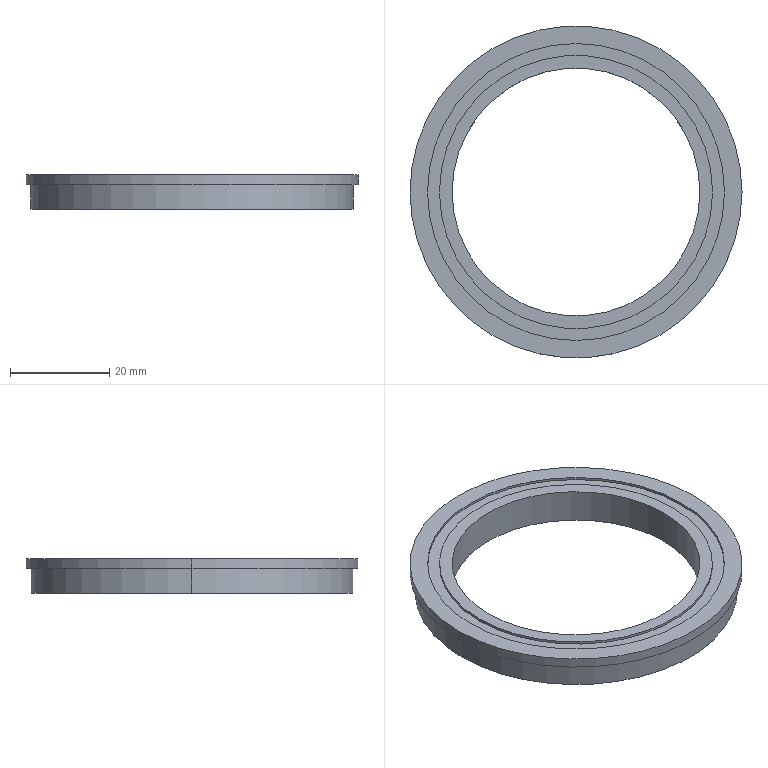Part | SolidWorks | features ICE 1, Revolution 1 | 1 solid | 21 faces | box 67 x 67 x 7 mm | volume 9465 mm3 | cylinder 14 | plane 7 | commonest cylinder face diameters 55.1 x4 59.9 x4 50 x2 65 x2 67 x2
STEP:
#1=CARTESIAN_POINT('',(33.5,0.,1.5));
#2=VERTEX_POINT('',#1);
#3=CARTESIAN_POINT('',(-33.5,0.,1.5));
#4=VERTEX_POINT('',#3);
#5=CARTESIAN_POINT('',(0.,0.,1.5));
#6=DIRECTION('',(0.,0.,1.));
#7=DIRECTION('',(1.,0.,0.));
#8=AXIS2_PLACEMENT_3D('',#5,#6,#7);
#9=CIRCLE('',#8,33.5);
#10=EDGE_CURVE('',#2,#4,#9,.T.);
#11=ORIENTED_EDGE('',*,*,#10,.T.);
#12=CARTESIAN_POINT('',(-33.5,0.,3.5));
#13=VERTEX_POINT('',#12);
#14=CARTESIAN_POINT('',(-33.5,0.,1.5));
#15=DIRECTION('',(0.,0.,1.));
#16=VECTOR('',#15,1000.);
#17=LINE('',#14,#16);
#18=EDGE_CURVE('',#4,#13,#17,.T.);
#19=ORIENTED_EDGE('',*,*,#18,.T.);
#20=CARTESIAN_POINT('',(33.5,0.,3.5));
#21=VERTEX_POINT('',#20);
#22=CARTESIAN_POINT('',(0.,0.,3.5));
#23=DIRECTION('',(0.,0.,1.));
#24=DIRECTION('',(1.,0.,0.));
#25=AXIS2_PLACEMENT_3D('',#22,#23,#24);
#26=CIRCLE('',#25,33.5);
#27=EDGE_CURVE('',#21,#13,#26,.T.);
#28=ORIENTED_EDGE('',*,*,#27,.F.);
#29=CARTESIAN_POINT('',(33.5,0.,1.5));
#30=DIRECTION('',(0.,0.,1.));
#31=VECTOR('',#30,1000.);
#32=LINE('',#29,#31);
#33=EDGE_CURVE('',#2,#21,#32,.T.);
#34=ORIENTED_EDGE('',*,*,#33,.F.);
#35=EDGE_LOOP('',(#11,#19,#28,#34));
#36=FACE_OUTER_BOUND('',#35,.T.);
#37=CARTESIAN_POINT('',(0.,0.,1.5));
#38=DIRECTION('',(0.,0.,1.));
#39=DIRECTION('',(1.,0.,0.));
#40=AXIS2_PLACEMENT_3D('',#37,#38,#39);
#41=CYLINDRICAL_SURFACE('',#40,33.5);
#42=ADVANCED_FACE('',(#36),#41,.T.);
#43=CARTESIAN_POINT('',(27.55,0.,-3.5));
#44=VERTEX_POINT('',#43);
#45=CARTESIAN_POINT('',(-27.55,0.,-3.5));
#46=VERTEX_POINT('',#45);
#47=CARTESIAN_POINT('',(0.,0.,-3.5));
#48=DIRECTION('',(0.,0.,1.));
#49=DIRECTION('',(1.,0.,0.));
#50=AXIS2_PLACEMENT_3D('',#47,#48,#49);
#51=CIRCLE('',#50,27.55);
#52=EDGE_CURVE('',#44,#46,#51,.T.);
#53=ORIENTED_EDGE('',*,*,#52,.T.);
#54=CARTESIAN_POINT('',(-27.55,0.,-3.));
#55=VERTEX_POINT('',#54);
#56=CARTESIAN_POINT('',(-27.55,0.,0.));
#57=DIRECTION('',(0.,0.,1.));
#58=VECTOR('',#57,1000.);
#59=LINE('',#56,#58);
#60=EDGE_CURVE('',#46,#55,#59,.T.);
#61=ORIENTED_EDGE('',*,*,#60,.T.);
#62=CARTESIAN_POINT('',(27.55,0.,-3.));
#63=VERTEX_POINT('',#62);
#64=CARTESIAN_POINT('',(0.,0.,-3.));
#65=DIRECTION('',(0.,0.,1.));
#66=DIRECTION('',(1.,0.,0.));
#67=AXIS2_PLACEMENT_3D('',#64,#65,#66);
#68=CIRCLE('',#67,27.55);
#69=EDGE_CURVE('',#63,#55,#68,.T.);
#70=ORIENTED_EDGE('',*,*,#69,.F.);
#71=CARTESIAN_POINT('',(27.55,0.,0.));
#72=DIRECTION('',(0.,0.,1.));
#73=VECTOR('',#72,1000.);
#74=LINE('',#71,#73);
#75=EDGE_CURVE('',#44,#63,#74,.T.);
#76=ORIENTED_EDGE('',*,*,#75,.F.);
#77=EDGE_LOOP('',(#53,#61,#70,#76));
#78=FACE_OUTER_BOUND('',#77,.T.);
#79=CARTESIAN_POINT('',(0.,0.,0.));
#80=DIRECTION('',(0.,0.,1.));
#81=DIRECTION('',(1.,0.,0.));
#82=AXIS2_PLACEMENT_3D('',#79,#80,#81);
#83=CYLINDRICAL_SURFACE('',#82,27.55);
#84=ADVANCED_FACE('',(#78),#83,.T.);
#85=CARTESIAN_POINT('',(-29.95,0.,-3.5));
#86=VERTEX_POINT('',#85);
#87=CARTESIAN_POINT('',(29.95,0.,-3.5));
#88=VERTEX_POINT('',#87);
#89=CARTESIAN_POINT('',(0.,0.,-3.5));
#90=DIRECTION('',(0.,0.,1.));
#91=DIRECTION('',(1.,0.,0.));
#92=AXIS2_PLACEMENT_3D('',#89,#90,#91);
#93=CIRCLE('',#92,29.95);
#94=EDGE_CURVE('',#86,#88,#93,.T.);
#95=ORIENTED_EDGE('',*,*,#94,.F.);
#96=CARTESIAN_POINT('',(-29.95,0.,-3.));
#97=VERTEX_POINT('',#96);
#98=CARTESIAN_POINT('',(-29.95,0.,0.));
#99=DIRECTION('',(0.,0.,1.));
#100=VECTOR('',#99,1000.);
#101=LINE('',#98,#100);
#102=EDGE_CURVE('',#86,#97,#101,.T.);
#103=ORIENTED_EDGE('',*,*,#102,.T.);
#104=CARTESIAN_POINT('',(29.95,0.,-3.));
#105=VERTEX_POINT('',#104);
#106=CARTESIAN_POINT('',(0.,0.,-3.));
#107=DIRECTION('',(0.,0.,1.));
#108=DIRECTION('',(1.,0.,0.));
#109=AXIS2_PLACEMENT_3D('',#106,#107,#108);
#110=CIRCLE('',#109,29.95);
#111=EDGE_CURVE('',#97,#105,#110,.T.);
#112=ORIENTED_EDGE('',*,*,#111,.T.);
#113=CARTESIAN_POINT('',(29.95,0.,0.));
#114=DIRECTION('',(0.,0.,1.));
#115=VECTOR('',#114,1000.);
#116=LINE('',#113,#115);
#117=EDGE_CURVE('',#88,#105,#116,.T.);
#118=ORIENTED_EDGE('',*,*,#117,.F.);
#119=EDGE_LOOP('',(#95,#103,#112,#118));
#120=FACE_OUTER_BOUND('',#119,.T.);
#121=CARTESIAN_POINT('',(0.,0.,0.));
#122=DIRECTION('',(0.,0.,1.));
#123=DIRECTION('',(1.,0.,0.));
#124=AXIS2_PLACEMENT_3D('',#121,#122,#123);
#125=CYLINDRICAL_SURFACE('',#124,29.95);
#126=ADVANCED_FACE('',(#120),#125,.F.);
#127=CARTESIAN_POINT('',(-29.95,0.,3.));
#128=VERTEX_POINT('',#127);
#129=CARTESIAN_POINT('',(29.95,0.,3.));
#130=VERTEX_POINT('',#129);
#131=CARTESIAN_POINT('',(0.,0.,3.));
#132=DIRECTION('',(0.,0.,1.));
#133=DIRECTION('',(1.,0.,0.));
#134=AXIS2_PLACEMENT_3D('',#131,#132,#133);
#135=CIRCLE('',#134,29.95);
#136=EDGE_CURVE('',#128,#130,#135,.T.);
#137=ORIENTED_EDGE('',*,*,#136,.F.);
#138=CARTESIAN_POINT('',(-29.95,0.,3.5));
#139=VERTEX_POINT('',#138);
#140=CARTESIAN_POINT('',(-29.95,0.,0.));
#141=DIRECTION('',(0.,0.,1.));
#142=VECTOR('',#141,1000.);
#143=LINE('',#140,#142);
#144=EDGE_CURVE('',#128,#139,#143,.T.);
#145=ORIENTED_EDGE('',*,*,#144,.T.);
#146=CARTESIAN_POINT('',(29.95,0.,3.5));
#147=VERTEX_POINT('',#146);
#148=CARTESIAN_POINT('',(0.,0.,3.5));
#149=DIRECTION('',(0.,0.,1.));
#150=DIRECTION('',(1.,0.,0.));
#151=AXIS2_PLACEMENT_3D('',#148,#149,#150);
#152=CIRCLE('',#151,29.95);
#153=EDGE_CURVE('',#139,#147,#152,.T.);
#154=ORIENTED_EDGE('',*,*,#153,.T.);
#155=CARTESIAN_POINT('',(29.95,0.,0.));
#156=DIRECTION('',(0.,0.,1.));
#157=VECTOR('',#156,1000.);
#158=LINE('',#155,#157);
#159=EDGE_CURVE('',#130,#147,#158,.T.);
#160=ORIENTED_EDGE('',*,*,#159,.F.);
#161=EDGE_LOOP('',(#137,#145,#154,#160));
#162=FACE_OUTER_BOUND('',#161,.T.);
#163=CARTESIAN_POINT('',(0.,0.,0.));
#164=DIRECTION('',(0.,0.,1.));
#165=DIRECTION('',(1.,0.,0.));
#166=AXIS2_PLACEMENT_3D('',#163,#164,#165);
#167=CYLINDRICAL_SURFACE('',#166,29.95);
#168=ADVANCED_FACE('',(#162),#167,.F.);
#169=CARTESIAN_POINT('',(27.55,0.,3.));
#170=VERTEX_POINT('',#169);
#171=CARTESIAN_POINT('',(-27.55,0.,3.));
#172=VERTEX_POINT('',#171);
#173=CARTESIAN_POINT('',(0.,0.,3.));
#174=DIRECTION('',(0.,0.,1.));
#175=DIRECTION('',(1.,0.,0.));
#176=AXIS2_PLACEMENT_3D('',#173,#174,#175);
#177=CIRCLE('',#176,27.55);
#178=EDGE_CURVE('',#170,#172,#177,.T.);
#179=ORIENTED_EDGE('',*,*,#178,.T.);
#180=CARTESIAN_POINT('',(-27.55,0.,3.5));
#181=VERTEX_POINT('',#180);
#182=CARTESIAN_POINT('',(-27.55,0.,0.));
#183=DIRECTION('',(0.,0.,1.));
#184=VECTOR('',#183,1000.);
#185=LINE('',#182,#184);
#186=EDGE_CURVE('',#172,#181,#185,.T.);
#187=ORIENTED_EDGE('',*,*,#186,.T.);
#188=CARTESIAN_POINT('',(27.55,0.,3.5));
#189=VERTEX_POINT('',#188);
#190=CARTESIAN_POINT('',(0.,0.,3.5));
#191=DIRECTION('',(0.,0.,1.));
#192=DIRECTION('',(1.,0.,0.));
#193=AXIS2_PLACEMENT_3D('',#190,#191,#192);
#194=CIRCLE('',#193,27.55);
#195=EDGE_CURVE('',#189,#181,#194,.T.);
#196=ORIENTED_EDGE('',*,*,#195,.F.);
#197=CARTESIAN_POINT('',(27.55,0.,0.));
#198=DIRECTION('',(0.,0.,1.));
#199=VECTOR('',#198,1000.);
#200=LINE('',#197,#199);
#201=EDGE_CURVE('',#170,#189,#200,.T.);
#202=ORIENTED_EDGE('',*,*,#201,.F.);
#203=EDGE_LOOP('',(#179,#187,#196,#202));
#204=FACE_OUTER_BOUND('',#203,.T.);
#205=CARTESIAN_POINT('',(0.,0.,0.));
#206=DIRECTION('',(0.,0.,1.));
#207=DIRECTION('',(1.,0.,0.));
#208=AXIS2_PLACEMENT_3D('',#205,#206,#207);
#209=CYLINDRICAL_SURFACE('',#208,27.55);
#210=ADVANCED_FACE('',(#204),#209,.T.);
#211=CARTESIAN_POINT('',(-25.,0.,-3.5));
#212=VERTEX_POINT('',#211);
#213=CARTESIAN_POINT('',(25.,0.,-3.5));
#214=VERTEX_POINT('',#213);
#215=CARTESIAN_POINT('',(0.,0.,-3.5));
#216=DIRECTION('',(0.,0.,1.));
#217=DIRECTION('',(1.,0.,0.));
#218=AXIS2_PLACEMENT_3D('',#215,#216,#217);
#219=CIRCLE('',#218,25.);
#220=EDGE_CURVE('',#212,#214,#219,.T.);
#221=ORIENTED_EDGE('',*,*,#220,.F.);
#222=CARTESIAN_POINT('',(-25.,0.,3.5));
#223=VERTEX_POINT('',#222);
#224=CARTESIAN_POINT('',(-25.,0.,0.));
#225=DIRECTION('',(0.,0.,1.));
#226=VECTOR('',#225,1000.);
#227=LINE('',#224,#226);
#228=EDGE_CURVE('',#212,#223,#227,.T.);
#229=ORIENTED_EDGE('',*,*,#228,.T.);
#230=CARTESIAN_POINT('',(25.,0.,3.5));
#231=VERTEX_POINT('',#230);
#232=CARTESIAN_POINT('',(0.,0.,3.5));
#233=DIRECTION('',(0.,0.,1.));
#234=DIRECTION('',(1.,0.,0.));
#235=AXIS2_PLACEMENT_3D('',#232,#233,#234);
#236=CIRCLE('',#235,25.);
#237=EDGE_CURVE('',#223,#231,#236,.T.);
#238=ORIENTED_EDGE('',*,*,#237,.T.);
#239=CARTESIAN_POINT('',(25.,0.,0.));
#240=DIRECTION('',(0.,0.,1.));
#241=VECTOR('',#240,1000.);
#242=LINE('',#239,#241);
#243=EDGE_CURVE('',#214,#231,#242,.T.);
#244=ORIENTED_EDGE('',*,*,#243,.F.);
#245=EDGE_LOOP('',(#221,#229,#238,#244));
#246=FACE_OUTER_BOUND('',#245,.T.);
#247=CARTESIAN_POINT('',(0.,0.,0.));
#248=DIRECTION('',(0.,0.,1.));
#249=DIRECTION('',(1.,0.,0.));
#250=AXIS2_PLACEMENT_3D('',#247,#248,#249);
#251=CYLINDRICAL_SURFACE('',#250,25.);
#252=ADVANCED_FACE('',(#246),#251,.F.);
#253=CARTESIAN_POINT('',(32.5,0.,-3.5));
#254=VERTEX_POINT('',#253);
#255=CARTESIAN_POINT('',(-32.5,0.,-3.5));
#256=VERTEX_POINT('',#255);
#257=CARTESIAN_POINT('',(0.,0.,-3.5));
#258=DIRECTION('',(0.,0.,1.));
#259=DIRECTION('',(1.,0.,0.));
#260=AXIS2_PLACEMENT_3D('',#257,#258,#259);
#261=CIRCLE('',#260,32.5);
#262=EDGE_CURVE('',#254,#256,#261,.T.);
#263=ORIENTED_EDGE('',*,*,#262,.T.);
#264=CARTESIAN_POINT('',(-32.5,0.,1.5));
#265=VERTEX_POINT('',#264);
#266=CARTESIAN_POINT('',(-32.5,0.,0.));
#267=DIRECTION('',(0.,0.,1.));
#268=VECTOR('',#267,1000.);
#269=LINE('',#266,#268);
#270=EDGE_CURVE('',#256,#265,#269,.T.);
#271=ORIENTED_EDGE('',*,*,#270,.T.);
#272=CARTESIAN_POINT('',(32.5,0.,1.5));
#273=VERTEX_POINT('',#272);
#274=CARTESIAN_POINT('',(0.,0.,1.5));
#275=DIRECTION('',(0.,0.,1.));
#276=DIRECTION('',(1.,0.,0.));
#277=AXIS2_PLACEMENT_3D('',#274,#275,#276);
#278=CIRCLE('',#277,32.5);
#279=EDGE_CURVE('',#273,#265,#278,.T.);
#280=ORIENTED_EDGE('',*,*,#279,.F.);
#281=CARTESIAN_POINT('',(32.5,0.,0.));
#282=DIRECTION('',(0.,0.,1.));
#283=VECTOR('',#282,1000.);
#284=LINE('',#281,#283);
#285=EDGE_CURVE('',#254,#273,#284,.T.);
#286=ORIENTED_EDGE('',*,*,#285,.F.);
#287=EDGE_LOOP('',(#263,#271,#280,#286));
#288=FACE_OUTER_BOUND('',#287,.T.);
#289=CARTESIAN_POINT('',(0.,0.,0.));
#290=DIRECTION('',(0.,0.,1.));
#291=DIRECTION('',(1.,0.,0.));
#292=AXIS2_PLACEMENT_3D('',#289,#290,#291);
#293=CYLINDRICAL_SURFACE('',#292,32.5);
#294=ADVANCED_FACE('',(#288),#293,.T.);
#295=ORIENTED_EDGE('',*,*,#270,.F.);
#296=CARTESIAN_POINT('',(0.,0.,-3.5));
#297=DIRECTION('',(0.,0.,1.));
#298=DIRECTION('',(1.,0.,0.));
#299=AXIS2_PLACEMENT_3D('',#296,#297,#298);
#300=CIRCLE('',#299,32.5);
#301=EDGE_CURVE('',#256,#254,#300,.T.);
#302=ORIENTED_EDGE('',*,*,#301,.T.);
#303=ORIENTED_EDGE('',*,*,#285,.T.);
#304=CARTESIAN_POINT('',(0.,0.,1.5));
#305=DIRECTION('',(0.,0.,1.));
#306=DIRECTION('',(1.,0.,0.));
#307=AXIS2_PLACEMENT_3D('',#304,#305,#306);
#308=CIRCLE('',#307,32.5);
#309=EDGE_CURVE('',#265,#273,#308,.T.);
#310=ORIENTED_EDGE('',*,*,#309,.F.);
#311=EDGE_LOOP('',(#295,#302,#303,#310));
#312=FACE_OUTER_BOUND('',#311,.T.);
#313=CARTESIAN_POINT('',(0.,0.,0.));
#314=DIRECTION('',(0.,0.,1.));
#315=DIRECTION('',(1.,0.,0.));
#316=AXIS2_PLACEMENT_3D('',#313,#314,#315);
#317=CYLINDRICAL_SURFACE('',#316,32.5);
#318=ADVANCED_FACE('',(#312),#317,.T.);
#319=ORIENTED_EDGE('',*,*,#228,.F.);
#320=CARTESIAN_POINT('',(0.,0.,-3.5));
#321=DIRECTION('',(0.,0.,1.));
#322=DIRECTION('',(1.,0.,0.));
#323=AXIS2_PLACEMENT_3D('',#320,#321,#322);
#324=CIRCLE('',#323,25.);
#325=EDGE_CURVE('',#214,#212,#324,.T.);
#326=ORIENTED_EDGE('',*,*,#325,.F.);
#327=ORIENTED_EDGE('',*,*,#243,.T.);
#328=CARTESIAN_POINT('',(0.,0.,3.5));
#329=DIRECTION('',(0.,0.,1.));
#330=DIRECTION('',(1.,0.,0.));
#331=AXIS2_PLACEMENT_3D('',#328,#329,#330);
#332=CIRCLE('',#331,25.);
#333=EDGE_CURVE('',#231,#223,#332,.T.);
#334=ORIENTED_EDGE('',*,*,#333,.T.);
#335=EDGE_LOOP('',(#319,#326,#327,#334));
#336=FACE_OUTER_BOUND('',#335,.T.);
#337=CARTESIAN_POINT('',(0.,0.,0.));
#338=DIRECTION('',(0.,0.,1.));
#339=DIRECTION('',(1.,0.,0.));
#340=AXIS2_PLACEMENT_3D('',#337,#338,#339);
#341=CYLINDRICAL_SURFACE('',#340,25.);
#342=ADVANCED_FACE('',(#336),#341,.F.);
#343=ORIENTED_EDGE('',*,*,#333,.F.);
#344=ORIENTED_EDGE('',*,*,#237,.F.);
#345=EDGE_LOOP('',(#343,#344));
#346=FACE_BOUND('',#345,.T.);
#347=ORIENTED_EDGE('',*,*,#195,.T.);
#348=CARTESIAN_POINT('',(0.,0.,3.5));
#349=DIRECTION('',(0.,0.,1.));
#350=DIRECTION('',(1.,0.,0.));
#351=AXIS2_PLACEMENT_3D('',#348,#349,#350);
#352=CIRCLE('',#351,27.55);
#353=EDGE_CURVE('',#181,#189,#352,.T.);
#354=ORIENTED_EDGE('',*,*,#353,.T.);
#355=EDGE_LOOP('',(#347,#354));
#356=FACE_OUTER_BOUND('',#355,.T.);
#357=CARTESIAN_POINT('',(0.,25.,3.5));
#358=DIRECTION('',(0.,0.,-1.));
#359=DIRECTION('',(-1.,0.,0.));
#360=AXIS2_PLACEMENT_3D('',#357,#358,#359);
#361=PLANE('',#360);
#362=ADVANCED_FACE('',(#346,#356),#361,.F.);
#363=ORIENTED_EDGE('',*,*,#186,.F.);
#364=CARTESIAN_POINT('',(0.,0.,3.));
#365=DIRECTION('',(0.,0.,1.));
#366=DIRECTION('',(1.,0.,0.));
#367=AXIS2_PLACEMENT_3D('',#364,#365,#366);
#368=CIRCLE('',#367,27.55);
#369=EDGE_CURVE('',#172,#170,#368,.T.);
#370=ORIENTED_EDGE('',*,*,#369,.T.);
#371=ORIENTED_EDGE('',*,*,#201,.T.);
#372=ORIENTED_EDGE('',*,*,#353,.F.);
#373=EDGE_LOOP('',(#363,#370,#371,#372));
#374=FACE_OUTER_BOUND('',#373,.T.);
#375=CARTESIAN_POINT('',(0.,0.,0.));
#376=DIRECTION('',(0.,0.,1.));
#377=DIRECTION('',(1.,0.,0.));
#378=AXIS2_PLACEMENT_3D('',#375,#376,#377);
#379=CYLINDRICAL_SURFACE('',#378,27.55);
#380=ADVANCED_FACE('',(#374),#379,.T.);
#381=ORIENTED_EDGE('',*,*,#178,.F.);
#382=ORIENTED_EDGE('',*,*,#369,.F.);
#383=EDGE_LOOP('',(#381,#382));
#384=FACE_BOUND('',#383,.T.);
#385=CARTESIAN_POINT('',(0.,0.,3.));
#386=DIRECTION('',(0.,0.,1.));
#387=DIRECTION('',(1.,0.,0.));
#388=AXIS2_PLACEMENT_3D('',#385,#386,#387);
#389=CIRCLE('',#388,29.95);
#390=EDGE_CURVE('',#130,#128,#389,.T.);
#391=ORIENTED_EDGE('',*,*,#390,.T.);
#392=ORIENTED_EDGE('',*,*,#136,.T.);
#393=EDGE_LOOP('',(#391,#392));
#394=FACE_OUTER_BOUND('',#393,.T.);
#395=CARTESIAN_POINT('',(0.,27.55,3.));
#396=DIRECTION('',(0.,0.,-1.));
#397=DIRECTION('',(-1.,0.,0.));
#398=AXIS2_PLACEMENT_3D('',#395,#396,#397);
#399=PLANE('',#398);
#400=ADVANCED_FACE('',(#384,#394),#399,.F.);
#401=ORIENTED_EDGE('',*,*,#144,.F.);
#402=ORIENTED_EDGE('',*,*,#390,.F.);
#403=ORIENTED_EDGE('',*,*,#159,.T.);
#404=CARTESIAN_POINT('',(0.,0.,3.5));
#405=DIRECTION('',(0.,0.,1.));
#406=DIRECTION('',(1.,0.,0.));
#407=AXIS2_PLACEMENT_3D('',#404,#405,#406);
#408=CIRCLE('',#407,29.95);
#409=EDGE_CURVE('',#147,#139,#408,.T.);
#410=ORIENTED_EDGE('',*,*,#409,.T.);
#411=EDGE_LOOP('',(#401,#402,#403,#410));
#412=FACE_OUTER_BOUND('',#411,.T.);
#413=CARTESIAN_POINT('',(0.,0.,0.));
#414=DIRECTION('',(0.,0.,1.));
#415=DIRECTION('',(1.,0.,0.));
#416=AXIS2_PLACEMENT_3D('',#413,#414,#415);
#417=CYLINDRICAL_SURFACE('',#416,29.95);
#418=ADVANCED_FACE('',(#412),#417,.F.);
#419=ORIENTED_EDGE('',*,*,#409,.F.);
#420=ORIENTED_EDGE('',*,*,#153,.F.);
#421=EDGE_LOOP('',(#419,#420));
#422=FACE_BOUND('',#421,.T.);
#423=ORIENTED_EDGE('',*,*,#27,.T.);
#424=CARTESIAN_POINT('',(0.,0.,3.5));
#425=DIRECTION('',(0.,0.,1.));
#426=DIRECTION('',(1.,0.,0.));
#427=AXIS2_PLACEMENT_3D('',#424,#425,#426);
#428=CIRCLE('',#427,33.5);
#429=EDGE_CURVE('',#13,#21,#428,.T.);
#430=ORIENTED_EDGE('',*,*,#429,.T.);
#431=EDGE_LOOP('',(#423,#430));
#432=FACE_OUTER_BOUND('',#431,.T.);
#433=CARTESIAN_POINT('',(0.,29.95,3.5));
#434=DIRECTION('',(0.,0.,-1.));
#435=DIRECTION('',(-1.,0.,0.));
#436=AXIS2_PLACEMENT_3D('',#433,#434,#435);
#437=PLANE('',#436);
#438=ADVANCED_FACE('',(#422,#432),#437,.F.);
#439=ORIENTED_EDGE('',*,*,#262,.F.);
#440=ORIENTED_EDGE('',*,*,#301,.F.);
#441=EDGE_LOOP('',(#439,#440));
#442=FACE_OUTER_BOUND('',#441,.T.);
#443=CARTESIAN_POINT('',(0.,0.,-3.5));
#444=DIRECTION('',(0.,0.,1.));
#445=DIRECTION('',(1.,0.,0.));
#446=AXIS2_PLACEMENT_3D('',#443,#444,#445);
#447=CIRCLE('',#446,29.95);
#448=EDGE_CURVE('',#88,#86,#447,.T.);
#449=ORIENTED_EDGE('',*,*,#448,.T.);
#450=ORIENTED_EDGE('',*,*,#94,.T.);
#451=EDGE_LOOP('',(#449,#450));
#452=FACE_BOUND('',#451,.T.);
#453=CARTESIAN_POINT('',(0.,29.95,-3.5));
#454=DIRECTION('',(0.,0.,1.));
#455=DIRECTION('',(1.,0.,0.));
#456=AXIS2_PLACEMENT_3D('',#453,#454,#455);
#457=PLANE('',#456);
#458=ADVANCED_FACE('',(#442,#452),#457,.F.);
#459=ORIENTED_EDGE('',*,*,#102,.F.);
#460=ORIENTED_EDGE('',*,*,#448,.F.);
#461=ORIENTED_EDGE('',*,*,#117,.T.);
#462=CARTESIAN_POINT('',(0.,0.,-3.));
#463=DIRECTION('',(0.,0.,1.));
#464=DIRECTION('',(1.,0.,0.));
#465=AXIS2_PLACEMENT_3D('',#462,#463,#464);
#466=CIRCLE('',#465,29.95);
#467=EDGE_CURVE('',#105,#97,#466,.T.);
#468=ORIENTED_EDGE('',*,*,#467,.T.);
#469=EDGE_LOOP('',(#459,#460,#461,#468));
#470=FACE_OUTER_BOUND('',#469,.T.);
#471=CARTESIAN_POINT('',(0.,0.,0.));
#472=DIRECTION('',(0.,0.,1.));
#473=DIRECTION('',(1.,0.,0.));
#474=AXIS2_PLACEMENT_3D('',#471,#472,#473);
#475=CYLINDRICAL_SURFACE('',#474,29.95);
#476=ADVANCED_FACE('',(#470),#475,.F.);
#477=ORIENTED_EDGE('',*,*,#467,.F.);
#478=ORIENTED_EDGE('',*,*,#111,.F.);
#479=EDGE_LOOP('',(#477,#478));
#480=FACE_OUTER_BOUND('',#479,.T.);
#481=ORIENTED_EDGE('',*,*,#69,.T.);
#482=CARTESIAN_POINT('',(0.,0.,-3.));
#483=DIRECTION('',(0.,0.,1.));
#484=DIRECTION('',(1.,0.,0.));
#485=AXIS2_PLACEMENT_3D('',#482,#483,#484);
#486=CIRCLE('',#485,27.55);
#487=EDGE_CURVE('',#55,#63,#486,.T.);
#488=ORIENTED_EDGE('',*,*,#487,.T.);
#489=EDGE_LOOP('',(#481,#488));
#490=FACE_BOUND('',#489,.T.);
#491=CARTESIAN_POINT('',(0.,27.55,-3.));
#492=DIRECTION('',(0.,0.,1.));
#493=DIRECTION('',(1.,0.,0.));
#494=AXIS2_PLACEMENT_3D('',#491,#492,#493);
#495=PLANE('',#494);
#496=ADVANCED_FACE('',(#480,#490),#495,.F.);
#497=ORIENTED_EDGE('',*,*,#60,.F.);
#498=CARTESIAN_POINT('',(0.,0.,-3.5));
#499=DIRECTION('',(0.,0.,1.));
#500=DIRECTION('',(1.,0.,0.));
#501=AXIS2_PLACEMENT_3D('',#498,#499,#500);
#502=CIRCLE('',#501,27.55);
#503=EDGE_CURVE('',#46,#44,#502,.T.);
#504=ORIENTED_EDGE('',*,*,#503,.T.);
#505=ORIENTED_EDGE('',*,*,#75,.T.);
#506=ORIENTED_EDGE('',*,*,#487,.F.);
#507=EDGE_LOOP('',(#497,#504,#505,#506));
#508=FACE_OUTER_BOUND('',#507,.T.);
#509=CARTESIAN_POINT('',(0.,0.,0.));
#510=DIRECTION('',(0.,0.,1.));
#511=DIRECTION('',(1.,0.,0.));
#512=AXIS2_PLACEMENT_3D('',#509,#510,#511);
#513=CYLINDRICAL_SURFACE('',#512,27.55);
#514=ADVANCED_FACE('',(#508),#513,.T.);
#515=ORIENTED_EDGE('',*,*,#52,.F.);
#516=ORIENTED_EDGE('',*,*,#503,.F.);
#517=EDGE_LOOP('',(#515,#516));
#518=FACE_OUTER_BOUND('',#517,.T.);
#519=ORIENTED_EDGE('',*,*,#325,.T.);
#520=ORIENTED_EDGE('',*,*,#220,.T.);
#521=EDGE_LOOP('',(#519,#520));
#522=FACE_BOUND('',#521,.T.);
#523=CARTESIAN_POINT('',(0.,25.,-3.5));
#524=DIRECTION('',(0.,0.,1.));
#525=DIRECTION('',(1.,0.,0.));
#526=AXIS2_PLACEMENT_3D('',#523,#524,#525);
#527=PLANE('',#526);
#528=ADVANCED_FACE('',(#518,#522),#527,.F.);
#529=ORIENTED_EDGE('',*,*,#18,.F.);
#530=CARTESIAN_POINT('',(0.,0.,1.5));
#531=DIRECTION('',(0.,0.,1.));
#532=DIRECTION('',(1.,0.,0.));
#533=AXIS2_PLACEMENT_3D('',#530,#531,#532);
#534=CIRCLE('',#533,33.5);
#535=EDGE_CURVE('',#4,#2,#534,.T.);
#536=ORIENTED_EDGE('',*,*,#535,.T.);
#537=ORIENTED_EDGE('',*,*,#33,.T.);
#538=ORIENTED_EDGE('',*,*,#429,.F.);
#539=EDGE_LOOP('',(#529,#536,#537,#538));
#540=FACE_OUTER_BOUND('',#539,.T.);
#541=CARTESIAN_POINT('',(0.,0.,1.5));
#542=DIRECTION('',(0.,0.,1.));
#543=DIRECTION('',(1.,0.,0.));
#544=AXIS2_PLACEMENT_3D('',#541,#542,#543);
#545=CYLINDRICAL_SURFACE('',#544,33.5);
#546=ADVANCED_FACE('',(#540),#545,.T.);
#547=ORIENTED_EDGE('',*,*,#279,.T.);
#548=ORIENTED_EDGE('',*,*,#309,.T.);
#549=EDGE_LOOP('',(#547,#548));
#550=FACE_BOUND('',#549,.T.);
#551=ORIENTED_EDGE('',*,*,#10,.F.);
#552=ORIENTED_EDGE('',*,*,#535,.F.);
#553=EDGE_LOOP('',(#551,#552));
#554=FACE_OUTER_BOUND('',#553,.T.);
#555=CARTESIAN_POINT('',(0.,0.,1.5));
#556=DIRECTION('',(0.,0.,1.));
#557=DIRECTION('',(1.,0.,0.));
#558=AXIS2_PLACEMENT_3D('',#555,#556,#557);
#559=PLANE('',#558);
#560=ADVANCED_FACE('',(#550,#554),#559,.F.);
#561=CLOSED_SHELL('',(#42,#84,#126,#168,#210,#252,#294,#318,#342,#362,#380,#400,#418,#438,#458,#476,#496,#514,#528,#546,#560));
#562=MANIFOLD_SOLID_BREP('',#561);
#563=CARTESIAN_POINT('',(0.,0.,0.));
#564=DIRECTION('',(0.,0.,1.));
#565=DIRECTION('',(1.,0.,0.));
#566=AXIS2_PLACEMENT_3D('',#563,#564,#565);
#567=(LENGTH_UNIT()NAMED_UNIT(*)SI_UNIT(.MILLI.,.METRE.));
#568=UNCERTAINTY_MEASURE_WITH_UNIT(LENGTH_MEASURE(0.00001),#567,'','');
#569=(NAMED_UNIT(*)PLANE_ANGLE_UNIT()SI_UNIT($,.RADIAN.));
#570=(NAMED_UNIT(*)SI_UNIT($,.STERADIAN.)SOLID_ANGLE_UNIT());
#571=(GEOMETRIC_REPRESENTATION_CONTEXT(3)GLOBAL_UNCERTAINTY_ASSIGNED_CONTEXT((#568))GLOBAL_UNIT_ASSIGNED_CONTEXT((#567,#569,#570))REPRESENTATION_CONTEXT('',''));
#572=ADVANCED_BREP_SHAPE_REPRESENTATION('',(#562,#566),#571);